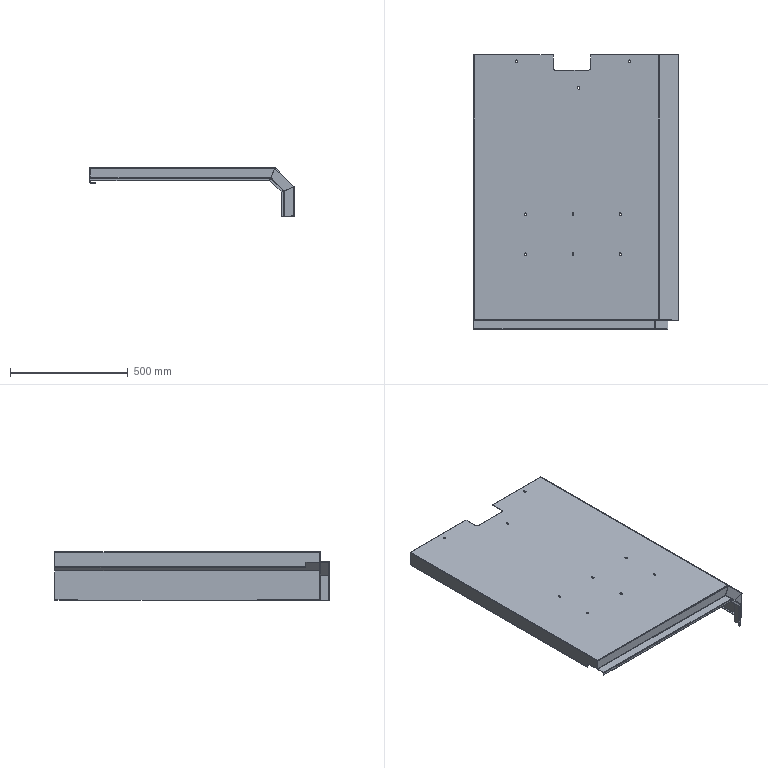Part | STEP file | Right Front | 1 solid | 163 faces | box 868 x 1166 x 207 mm | volume 2658932 mm3 | plane 98 | cylinder 57 | spline 8 | commonest cylinder face diameters 1 x22 7 x18 5 x15 20 x2